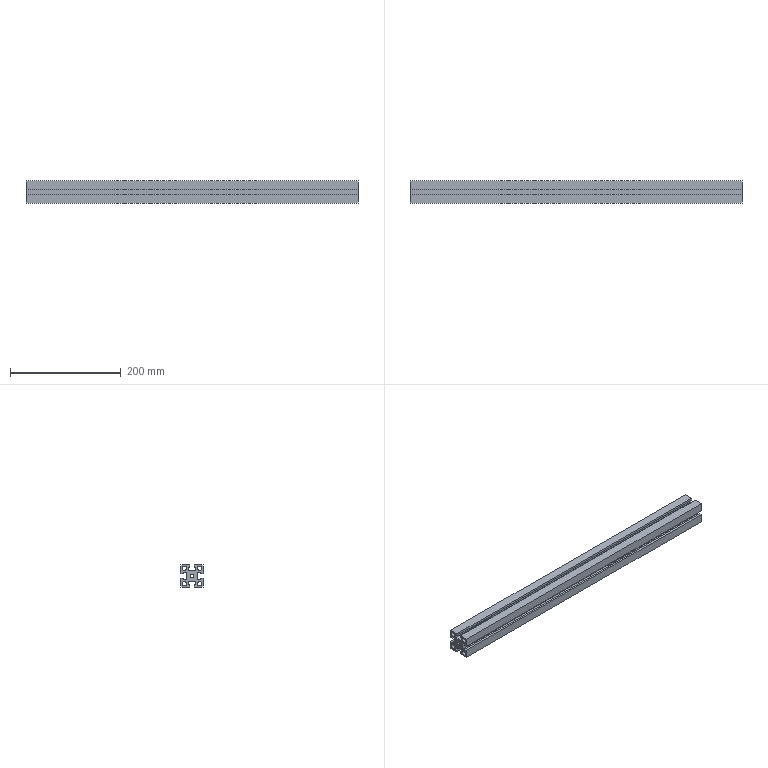Part | STEP file | 1 solid | 48 faces | box 600 x 40 x 40 mm | volume 535009 mm3 | plane 38 | cylinder 10 | commonest cylinder face diameters 8 x8 6.7 x2